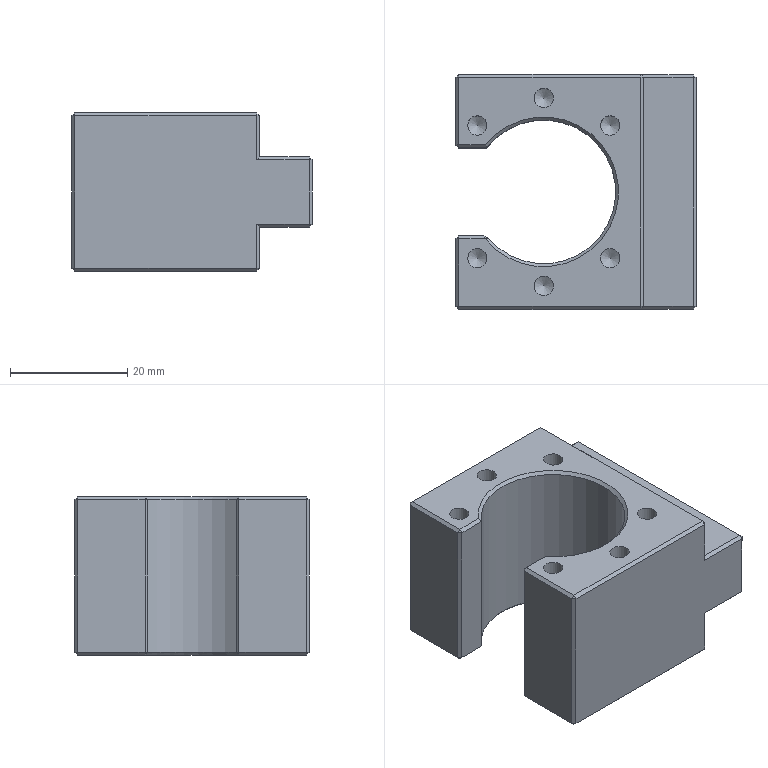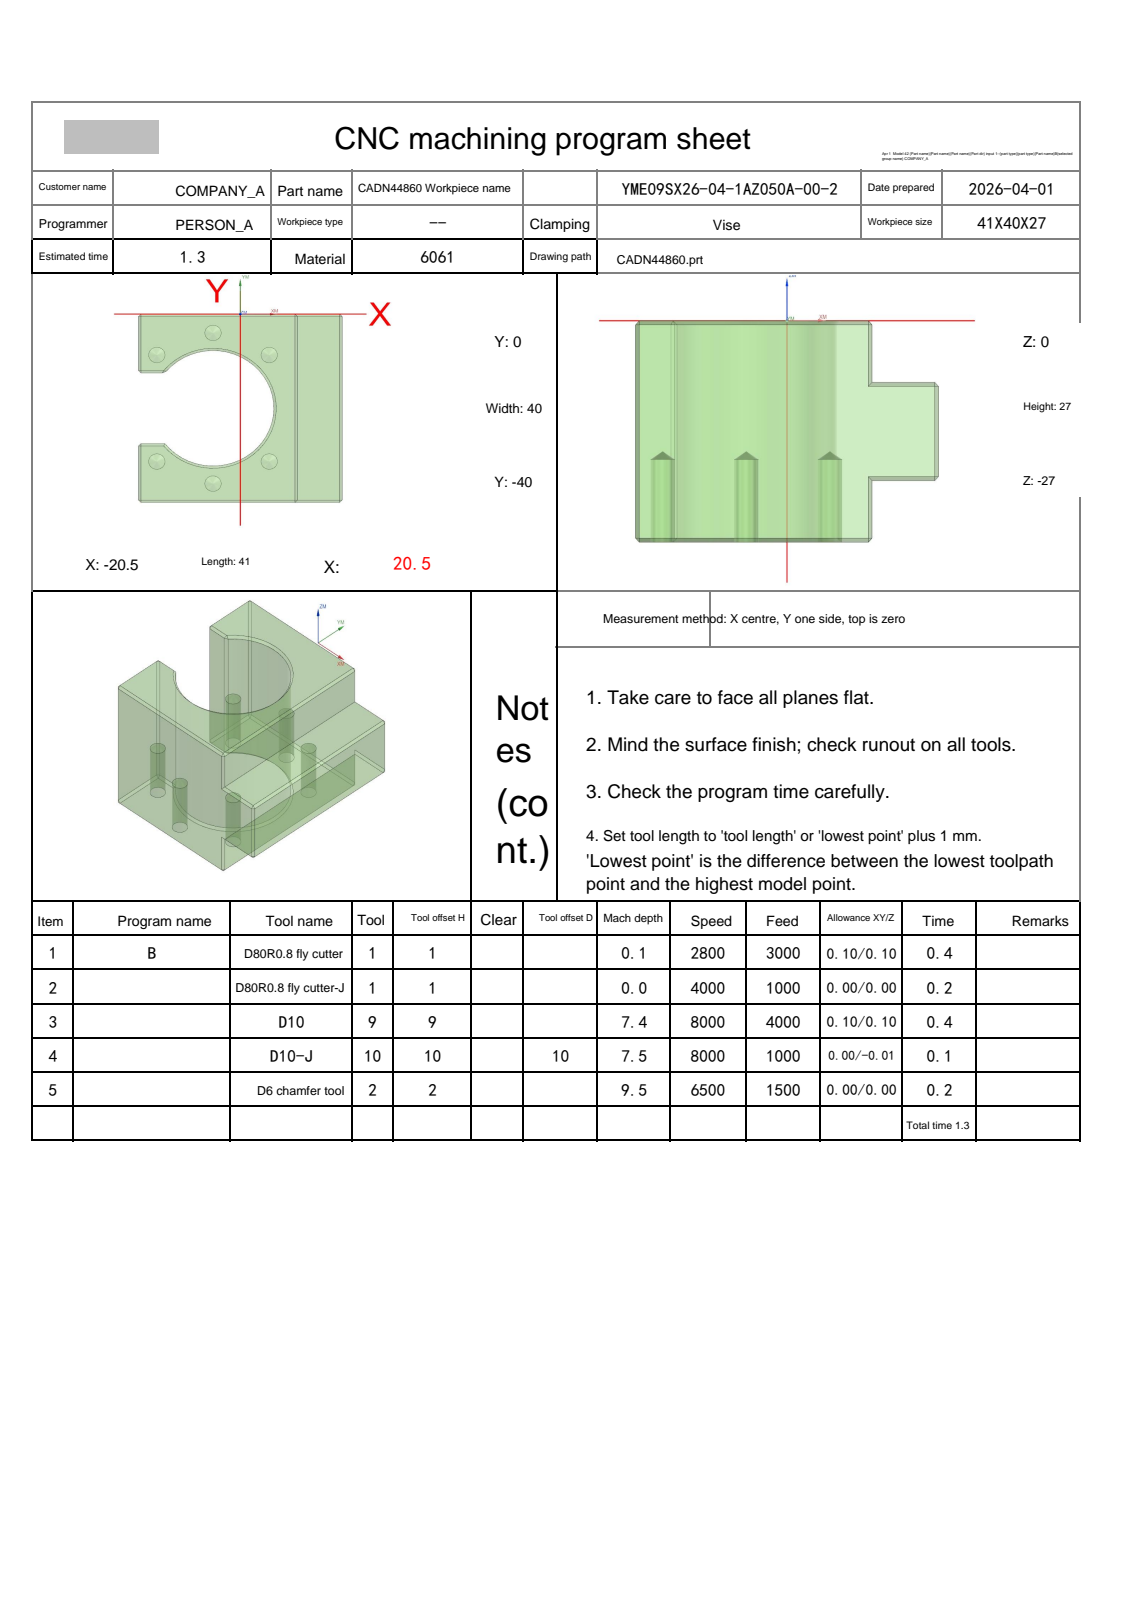NC program | NX | posted by the shop | part box 41 x 40 x 27 mm
Whole program:
%
O0001
(Machine time: 2.29 MIN)
(===Total Tool:4===)
(T1=D80R0.8 fly cutter  D=80.  R=0.8  D-  H01 Z=-0.   )
(T9=D10     D=10.  R=0.   D-  H09 Z=-7.4  )
(T10=D10-J  D=10.  R=0.   D10 H10 Z=-7.51 )
(T2=D6 chamfer tool   D=6.   R=0.   D-  H02 Z=-9.5  )
G80 G90 G17 G49 G40
G91 G28 Z0
M01
N1 T01 M06
(D80R0.8 fly cutter D=80. R=0.8 H=01 ce=0.10 di=0.10)
G00 G90 G54 X72.597 Y-20. M03 S2800
G43 H01 Z50.
M08
Z4.517
G01 Z2.517 F3000.
X60.597
X-60.597
X-72.597
Z4.517
G00 X72.597
Z4.033
G01 Z2.033
X60.597
X-60.597
X-72.597
Z4.033
G00 X72.597
Z3.55
G01 Z1.55
X60.597
X-60.597
X-72.597
Z3.55
G00 X72.597
Z3.067
G01 Z1.067
X60.597
X-60.597
X-72.597
Z3.067
G00 Z50.
X72.597
Z2.583
G01 Z.583
X60.597
X-60.597
X-72.597
Z2.583
G00 Z50.
X72.597
Z2.1
G01 Z.1
X60.597
X-60.597
X-72.597
Z2.1
G00 Z50.
G91 G28 Z0.0
M05
M09
G91 G28 Z0.0
M01
N2 T01 M06
(D80R0.8 fly cutter-J D=80. R=0.8 H=01 ce=0.00 di=0.00)
G00 G90 G54 X72.499 Y-20. M03 S4000
G43 H01 Z50.
M08
Z2.
G01 Z0.0 F1000.
X60.499
X-60.499
X-72.499
Z2.
G00 Z50.
G91 G28 Z0.0
M05
M09
G91 G28 Z0.0
M01
N3 T09 M06
(D10  D=10. R=0. H=09 ce=0.10 di=0.10)
G00 G90 G54 X22.322 Y-47.5 M03 S8000
G43 H09 Z12.8
M08
Z.931
G01 Z-.569 F4000.
X23.563 Y-44.4
G03 X24.1 Y-41.612 I-6.963 J2.788
G01 Y1.612
G03 X23.768 Y3.82 I-7.5 J0.0
X23. Y4.507 I-.956 J-.295
G01 X14.707 Y6.089
X14.52 Y6.107
G03 X13.52 Y5.107 I0.0 J-1.
X13.812 Y4.4 I1. J0.0
G01 X16.6 Y1.612
Y-41.612
X13.812 Y-44.4
X10.112 Y-48.1
Z.931
G00 X22.322 Y-47.5
Z.362
G01 Z-1.138
X23.563 Y-44.4
G03 X24.1 Y-41.612 I-6.963 J2.788
G01 Y1.612
G03 X23.768 Y3.82 I-7.5 J0.0
X23. Y4.507 I-.956 J-.295
G01 X14.707 Y6.089
X14.52 Y6.107
G03 X13.52 Y5.107 I0.0 J-1.
X13.812 Y4.4 I1. J0.0
G01 X16.6 Y1.612
Y-41.612
X13.812 Y-44.4
X10.112 Y-48.1
Z.362
G00 X22.322 Y-47.5
Z-.208
G01 Z-1.708
X23.563 Y-44.4
G03 X24.1 Y-41.612 I-6.963 J2.788
G01 Y1.612
G03 X23.768 Y3.82 I-7.5 J0.0
X23. Y4.507 I-.956 J-.295
G01 X14.707 Y6.089
X14.52 Y6.107
G03 X13.52 Y5.107 I0.0 J-1.
X13.812 Y4.4 I1. J0.0
G01 X16.6 Y1.612
Y-41.612
X13.812 Y-44.4
X10.112 Y-48.1
Z-.208
G00 X22.322 Y-47.5
Z-.777
G01 Z-2.277
X23.563 Y-44.4
G03 X24.1 Y-41.612 I-6.963 J2.788
G01 Y1.612
G03 X23.768 Y3.82 I-7.5 J0.0
X23. Y4.507 I-.956 J-.295
G01 X14.707 Y6.089
X14.52 Y6.107
G03 X13.52 Y5.107 I0.0 J-1.
X13.812 Y4.4 I1. J0.0
G01 X16.6 Y1.612
Y-41.612
X13.812 Y-44.4
X10.112 Y-48.1
Z-.777
G00 X22.322 Y-47.5
Z-1.346
G01 Z-2.846
X23.563 Y-44.4
G03 X24.1 Y-41.612 I-6.963 J2.788
G01 Y1.612
G03 X23.768 Y3.82 I-7.5 J0.0
X23. Y4.507 I-.956 J-.295
G01 X14.707 Y6.089
X14.52 Y6.107
G03 X13.52 Y5.107 I0.0 J-1.
X13.812 Y4.4 I1. J0.0
G01 X16.6 Y1.612
Y-41.612
X13.812 Y-44.4
X10.112 Y-48.1
Z-1.346
G00 X22.322 Y-47.5
Z-1.915
G01 Z-3.415
X23.563 Y-44.4
G03 X24.1 Y-41.612 I-6.963 J2.788
G01 Y1.612
G03 X23.768 Y3.82 I-7.5 J0.0
X23. Y4.507 I-.956 J-.295
G01 X14.707 Y6.089
X14.52 Y6.107
G03 X13.52 Y5.107 I0.0 J-1.
X13.812 Y4.4 I1. J0.0
G01 X16.6 Y1.612
Y-41.612
X13.812 Y-44.4
X10.112 Y-48.1
Z-1.915
G00 X22.322 Y-47.5
Z-2.485
G01 Z-3.985
X23.563 Y-44.4
G03 X24.1 Y-41.612 I-6.963 J2.788
G01 Y1.612
G03 X23.768 Y3.82 I-7.5 J0.0
X23. Y4.507 I-.956 J-.295
G01 X14.707 Y6.089
X14.52 Y6.107
G03 X13.52 Y5.107 I0.0 J-1.
X13.812 Y4.4 I1. J0.0
G01 X16.6 Y1.612
Y-41.612
X13.812 Y-44.4
X10.112 Y-48.1
Z-2.485
G00 X22.322 Y-47.5
Z-3.054
G01 Z-4.554
X23.563 Y-44.4
G03 X24.1 Y-41.612 I-6.963 J2.788
G01 Y1.612
G03 X23.768 Y3.82 I-7.5 J0.0
X23. Y4.507 I-.956 J-.295
G01 X14.707 Y6.089
X14.52 Y6.107
G03 X13.52 Y5.107 I0.0 J-1.
X13.812 Y4.4 I1. J0.0
G01 X16.6 Y1.612
Y-41.612
X13.812 Y-44.4
X10.112 Y-48.1
Z-3.054
G00 X22.322 Y-47.5
Z-3.623
G01 Z-5.123
X23.563 Y-44.4
G03 X24.1 Y-41.612 I-6.963 J2.788
G01 Y1.612
G03 X23.768 Y3.82 I-7.5 J0.0
X23. Y4.507 I-.956 J-.295
G01 X14.707 Y6.089
X14.52 Y6.107
G03 X13.52 Y5.107 I0.0 J-1.
X13.812 Y4.4 I1. J0.0
G01 X16.6 Y1.612
Y-41.612
X13.812 Y-44.4
X10.112 Y-48.1
Z-3.623
G00 X22.322 Y-47.5
Z-4.192
G01 Z-5.692
X23.563 Y-44.4
G03 X24.1 Y-41.612 I-6.963 J2.788
G01 Y1.612
G03 X23.768 Y3.82 I-7.5 J0.0
X23. Y4.507 I-.956 J-.295
G01 X14.707 Y6.089
X14.52 Y6.107
G03 X13.52 Y5.107 I0.0 J-1.
X13.812 Y4.4 I1. J0.0
G01 X16.6 Y1.612
Y-41.612
X13.812 Y-44.4
X10.112 Y-48.1
Z-4.192
G00 X22.322 Y-47.5
Z-4.762
G01 Z-6.262
X23.563 Y-44.4
G03 X24.1 Y-41.612 I-6.963 J2.788
G01 Y1.612
G03 X23.768 Y3.82 I-7.5 J0.0
X23. Y4.507 I-.956 J-.295
G01 X14.707 Y6.089
X14.52 Y6.107
G03 X13.52 Y5.107 I0.0 J-1.
X13.812 Y4.4 I1. J0.0
G01 X16.6 Y1.612
Y-41.612
X13.812 Y-44.4
X10.112 Y-48.1
Z-4.762
G00 X22.322 Y-47.5
Z-5.331
G01 Z-6.831
X23.563 Y-44.4
G03 X24.1 Y-41.612 I-6.963 J2.788
G01 Y1.612
G03 X23.768 Y3.82 I-7.5 J0.0
X23. Y4.507 I-.956 J-.295
G01 X14.707 Y6.089
X14.52 Y6.107
G03 X13.52 Y5.107 I0.0 J-1.
X13.812 Y4.4 I1. J0.0
G01 X16.6 Y1.612
Y-41.612
X13.812 Y-44.4
X10.112 Y-48.1
Z-5.331
G00 X22.322 Y-47.5
Z-5.9
G01 Z-7.4
X23.563 Y-44.4
G03 X24.1 Y-41.612 I-6.963 J2.788
G01 Y1.612
G03 X23.768 Y3.82 I-7.5 J0.0
X23. Y4.507 I-.956 J-.295
G01 X14.707 Y6.089
X14.52 Y6.107
G03 X13.52 Y5.107 I0.0 J-1.
X13.812 Y4.4 I1. J0.0
G01 X16.6 Y1.612
Y-41.612
X13.812 Y-44.4
X10.112 Y-48.1
Z-5.9
G00 Z12.8
G91 G28 Z0.0
M05
M09
G91 G28 Z0.0
M01
N4 T10 M06
(D10-J  D=10. R=0. H=10 ce=0.00 di=-0.01)
G00 G90 G54 X18.7 Y6.5 M03 S8000
G43 H10 Z12.8
M08
Z-6.5
G01 Z-7.51 F1000.
G41 D10
X18.5
G03 X16.5 Y4.5 I0.0 J-2.
G01 Y-44.5
G03 X18.5 Y-46.5 I2. J0.0
G01 G40 X18.7
Z-6.5
G00 Z12.8
G00 G90 X14.544 Y5.684 M03 S8000
Z7.8
Z-6.5
G01 Z-7.5 F1000.
G41 D10
X14.42 Y5.527
G03 X14.096 Y4.596 I1.176 J-.931
X14.536 Y3.536 I1.5 J0.0
G01 X15.036 Y3.036
G02 X16.5 Y-.5 I-3.536 J-3.536
G01 Y-39.5
G02 X15.036 Y-43.036 I-5. J0.0
G01 X14.536 Y-43.536
G03 X14.096 Y-44.596 I1.061 J-1.061
X14.42 Y-45.527 I1.5 J0.0
G01 G40 X14.544 Y-45.684
Z-6.5
G00 Z7.8
G91 G28 Z0.0
M05
M09
G91 G28 Z0.0
M01
N5 T02 M06
(D6 chamfer tool D=6. R=0. H=02 ce=0.00 di=0.00)
G00 G90 G54 X-14.087 Y-26.521 M03 S6500
G43 H02 Z50.
M08
Z2.001
G01 Z-1.999 F1500.
X-13.871 Y-26.745
G03 X-5.5 Y-30.75 I8.371 J6.745
X5.25 Y-20. I0.0 J10.75
X-5.5 Y-9.25 I-10.75 J0.0
X-13.871 Y-13.255 I0.0 J-10.75
G02 X-15.428 Y-14. I-1.557 J1.255
G01 X-20.
G02 X-22. Y-12. I0.0 J2.
G01 Y-.5
G02 X-20. Y1.5 I2. J0.0
G01 X11.
G02 X13. Y-.5 I0.0 J-2.
G01 Y-20.
Y-39.5
G02 X11. Y-41.5 I-2. J0.0
G01 X-20.
G02 X-22. Y-39.5 I0.0 J2.
G01 Y-28.
G02 X-20. Y-26. I2. J0.0
G01 X-15.428
X-15.073 Y-26.032
Z2.001
G00 Z10.
X13.897 Y1.613
Z-2.127
G01 Z-9.499
X13.961 Y1.552
X14.04 Y1.513
X14.061 Y1.494
X14.09 Y1.5
X20.
G02 X22. Y-.5 I0.0 J-2.
G01 Y-39.5
G02 X20. Y-41.5 I-2. J0.0
G01 X14.09
X14.061 Y-41.494
X14.04 Y-41.513
X13.961 Y-41.552
X13.897 Y-41.613
Z-2.127
G00 Z50.
M05
M09
G91 G28 Z0.0
G91 G28 Y0.0
M30
%